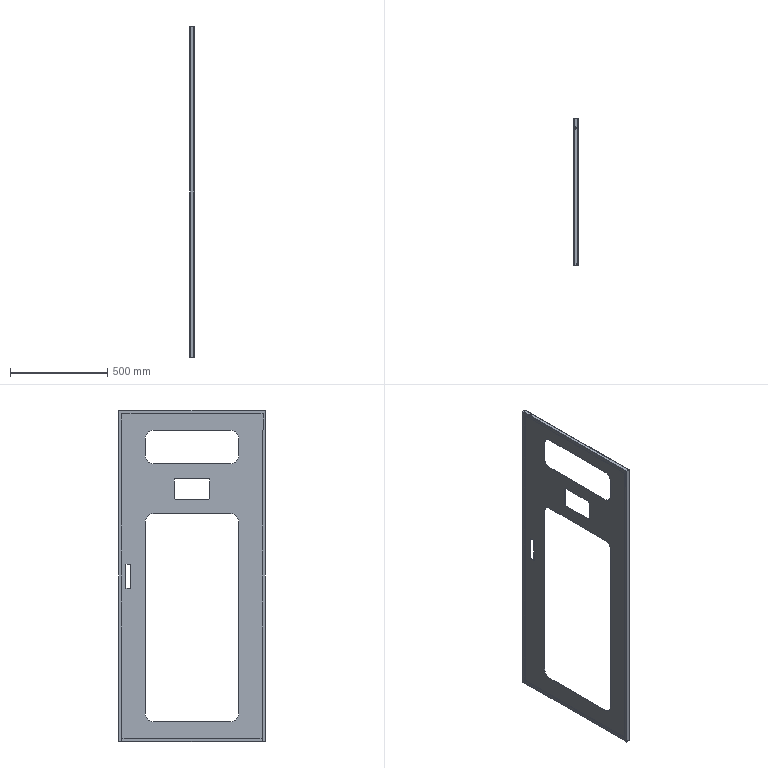Part | STEP file | RJWD-DY-0102_X2_5DE667DC95E8_17 | 1 solid | 190 faces | box 21 x 756.2 x 1704 mm | volume 844463 mm3 | plane 116 | cylinder 74 | commonest cylinder face diameters 3 x38 0.4 x8 2.4 x8 80 x8 9 x4 20.2 x4